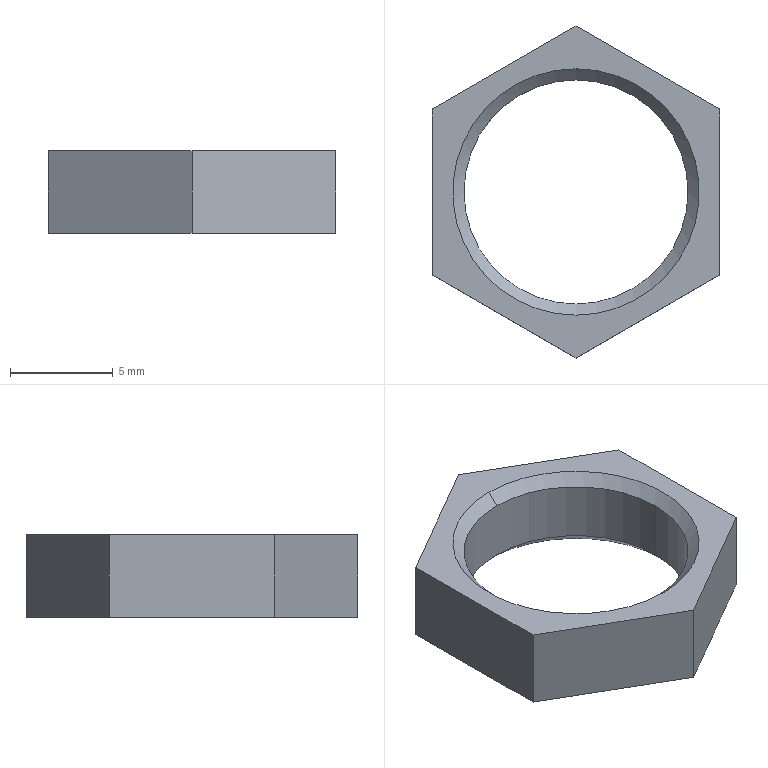Part | SolidWorks | features BaseBody 1 | 1 solid | 14 faces | box 14 x 16.166 x 4 mm | volume 294.157 mm3 | plane 8 | cone 4 | cylinder 2 | commonest cylinder face diameters 10.917 x2
STEP:
#1=CARTESIAN_POINT('',(-5.458,0.,-16.459));
#2=VERTEX_POINT('',#1);
#3=CARTESIAN_POINT('',(5.458,0.,-16.459));
#4=VERTEX_POINT('',#3);
#5=CARTESIAN_POINT('',(0.,0.,-16.459));
#6=DIRECTION('',(0.,0.,1.));
#7=DIRECTION('',(1.,0.,0.));
#8=AXIS2_PLACEMENT_3D('',#5,#6,#7);
#9=CIRCLE('',#8,5.458);
#10=EDGE_CURVE('',#2,#4,#9,.T.);
#11=ORIENTED_EDGE('',*,*,#10,.F.);
#12=CARTESIAN_POINT('',(-5.458,0.,-13.541));
#13=VERTEX_POINT('',#12);
#14=CARTESIAN_POINT('',(-5.458,0.,-50.));
#15=DIRECTION('',(0.,0.,1.));
#16=VECTOR('',#15,1000.);
#17=LINE('',#14,#16);
#18=EDGE_CURVE('',#2,#13,#17,.T.);
#19=ORIENTED_EDGE('',*,*,#18,.T.);
#20=CARTESIAN_POINT('',(0.,-5.458,-13.541));
#21=VERTEX_POINT('',#20);
#22=CARTESIAN_POINT('',(0.,0.,-13.541));
#23=DIRECTION('',(0.,0.,-1.));
#24=DIRECTION('',(1.,0.,0.));
#25=AXIS2_PLACEMENT_3D('',#22,#23,#24);
#26=CIRCLE('',#25,5.458);
#27=EDGE_CURVE('',#21,#13,#26,.T.);
#28=ORIENTED_EDGE('',*,*,#27,.F.);
#29=CARTESIAN_POINT('',(5.458,0.,-13.541));
#30=VERTEX_POINT('',#29);
#31=CARTESIAN_POINT('',(0.,0.,-13.541));
#32=DIRECTION('',(0.,0.,-1.));
#33=DIRECTION('',(1.,0.,0.));
#34=AXIS2_PLACEMENT_3D('',#31,#32,#33);
#35=CIRCLE('',#34,5.458);
#36=EDGE_CURVE('',#30,#21,#35,.T.);
#37=ORIENTED_EDGE('',*,*,#36,.F.);
#38=CARTESIAN_POINT('',(5.458,0.,-50.));
#39=DIRECTION('',(0.,0.,1.));
#40=VECTOR('',#39,1000.);
#41=LINE('',#38,#40);
#42=EDGE_CURVE('',#4,#30,#41,.T.);
#43=ORIENTED_EDGE('',*,*,#42,.F.);
#44=EDGE_LOOP('',(#11,#19,#28,#37,#43));
#45=FACE_OUTER_BOUND('',#44,.T.);
#46=CARTESIAN_POINT('',(0.,0.,-50.));
#47=DIRECTION('',(0.,0.,1.));
#48=DIRECTION('',(1.,0.,0.));
#49=AXIS2_PLACEMENT_3D('',#46,#47,#48);
#50=CYLINDRICAL_SURFACE('',#49,5.458);
#51=ADVANCED_FACE('',(#45),#50,.F.);
#52=ORIENTED_EDGE('',*,*,#27,.T.);
#53=CARTESIAN_POINT('',(0.,5.458,-13.541));
#54=VERTEX_POINT('',#53);
#55=CARTESIAN_POINT('',(0.,0.,-13.541));
#56=DIRECTION('',(0.,0.,-1.));
#57=DIRECTION('',(1.,0.,0.));
#58=AXIS2_PLACEMENT_3D('',#55,#56,#57);
#59=CIRCLE('',#58,5.458);
#60=EDGE_CURVE('',#13,#54,#59,.T.);
#61=ORIENTED_EDGE('',*,*,#60,.T.);
#62=CARTESIAN_POINT('',(0.,6.,-13.));
#63=VERTEX_POINT('',#62);
#64=CARTESIAN_POINT('',(0.,6.,-13.));
#65=DIRECTION('',(0.,0.7071,0.7071));
#66=VECTOR('',#65,1000.);
#67=LINE('',#64,#66);
#68=EDGE_CURVE('',#54,#63,#67,.T.);
#69=ORIENTED_EDGE('',*,*,#68,.T.);
#70=CARTESIAN_POINT('',(0.,-6.,-13.));
#71=VERTEX_POINT('',#70);
#72=CARTESIAN_POINT('',(0.,0.,-13.));
#73=DIRECTION('',(0.,0.,-1.));
#74=DIRECTION('',(0.,-1.,0.));
#75=AXIS2_PLACEMENT_3D('',#72,#73,#74);
#76=CIRCLE('',#75,6.);
#77=EDGE_CURVE('',#71,#63,#76,.T.);
#78=ORIENTED_EDGE('',*,*,#77,.F.);
#79=CARTESIAN_POINT('',(0.,-6.,-13.));
#80=DIRECTION('',(0.,-0.7071,0.7071));
#81=VECTOR('',#80,1000.);
#82=LINE('',#79,#81);
#83=EDGE_CURVE('',#21,#71,#82,.T.);
#84=ORIENTED_EDGE('',*,*,#83,.F.);
#85=EDGE_LOOP('',(#52,#61,#69,#78,#84));
#86=FACE_OUTER_BOUND('',#85,.T.);
#87=CARTESIAN_POINT('',(0.,0.,-13.));
#88=DIRECTION('',(0.,0.,1.));
#89=DIRECTION('',(0.,-1.,0.));
#90=AXIS2_PLACEMENT_3D('',#87,#88,#89);
#91=CONICAL_SURFACE('',#90,6.,0.7854);
#92=ADVANCED_FACE('',(#86),#91,.F.);
#93=ORIENTED_EDGE('',*,*,#10,.T.);
#94=CARTESIAN_POINT('',(6.,0.,-17.));
#95=VERTEX_POINT('',#94);
#96=CARTESIAN_POINT('',(6.,0.,-17.));
#97=DIRECTION('',(0.7071,0.,-0.7071));
#98=VECTOR('',#97,1000.);
#99=LINE('',#96,#98);
#100=EDGE_CURVE('',#4,#95,#99,.T.);
#101=ORIENTED_EDGE('',*,*,#100,.T.);
#102=CARTESIAN_POINT('',(-6.,0.,-17.));
#103=VERTEX_POINT('',#102);
#104=CARTESIAN_POINT('',(0.,0.,-17.));
#105=DIRECTION('',(0.,0.,1.));
#106=DIRECTION('',(-1.,0.,0.));
#107=AXIS2_PLACEMENT_3D('',#104,#105,#106);
#108=CIRCLE('',#107,6.);
#109=EDGE_CURVE('',#103,#95,#108,.T.);
#110=ORIENTED_EDGE('',*,*,#109,.F.);
#111=CARTESIAN_POINT('',(-6.,0.,-17.));
#112=DIRECTION('',(-0.7071,0.,-0.7071));
#113=VECTOR('',#112,1000.);
#114=LINE('',#111,#113);
#115=EDGE_CURVE('',#2,#103,#114,.T.);
#116=ORIENTED_EDGE('',*,*,#115,.F.);
#117=EDGE_LOOP('',(#93,#101,#110,#116));
#118=FACE_OUTER_BOUND('',#117,.T.);
#119=CARTESIAN_POINT('',(0.,0.,-17.));
#120=DIRECTION('',(0.,0.,-1.));
#121=DIRECTION('',(-1.,0.,0.));
#122=AXIS2_PLACEMENT_3D('',#119,#120,#121);
#123=CONICAL_SURFACE('',#122,6.,0.7854);
#124=ADVANCED_FACE('',(#118),#123,.F.);
#125=ORIENTED_EDGE('',*,*,#18,.F.);
#126=CARTESIAN_POINT('',(0.,0.,-16.459));
#127=DIRECTION('',(0.,0.,1.));
#128=DIRECTION('',(1.,0.,0.));
#129=AXIS2_PLACEMENT_3D('',#126,#127,#128);
#130=CIRCLE('',#129,5.458);
#131=EDGE_CURVE('',#4,#2,#130,.T.);
#132=ORIENTED_EDGE('',*,*,#131,.F.);
#133=ORIENTED_EDGE('',*,*,#42,.T.);
#134=CARTESIAN_POINT('',(0.,0.,-13.541));
#135=DIRECTION('',(0.,0.,-1.));
#136=DIRECTION('',(1.,0.,0.));
#137=AXIS2_PLACEMENT_3D('',#134,#135,#136);
#138=CIRCLE('',#137,5.458);
#139=EDGE_CURVE('',#54,#30,#138,.T.);
#140=ORIENTED_EDGE('',*,*,#139,.F.);
#141=ORIENTED_EDGE('',*,*,#60,.F.);
#142=EDGE_LOOP('',(#125,#132,#133,#140,#141));
#143=FACE_OUTER_BOUND('',#142,.T.);
#144=CARTESIAN_POINT('',(0.,0.,-50.));
#145=DIRECTION('',(0.,0.,1.));
#146=DIRECTION('',(1.,0.,0.));
#147=AXIS2_PLACEMENT_3D('',#144,#145,#146);
#148=CYLINDRICAL_SURFACE('',#147,5.458);
#149=ADVANCED_FACE('',(#143),#148,.F.);
#150=ORIENTED_EDGE('',*,*,#68,.F.);
#151=ORIENTED_EDGE('',*,*,#139,.T.);
#152=ORIENTED_EDGE('',*,*,#36,.T.);
#153=ORIENTED_EDGE('',*,*,#83,.T.);
#154=CARTESIAN_POINT('',(0.,0.,-13.));
#155=DIRECTION('',(0.,0.,-1.));
#156=DIRECTION('',(0.,-1.,0.));
#157=AXIS2_PLACEMENT_3D('',#154,#155,#156);
#158=CIRCLE('',#157,6.);
#159=EDGE_CURVE('',#63,#71,#158,.T.);
#160=ORIENTED_EDGE('',*,*,#159,.F.);
#161=EDGE_LOOP('',(#150,#151,#152,#153,#160));
#162=FACE_OUTER_BOUND('',#161,.T.);
#163=CARTESIAN_POINT('',(0.,0.,-13.));
#164=DIRECTION('',(0.,0.,1.));
#165=DIRECTION('',(0.,-1.,0.));
#166=AXIS2_PLACEMENT_3D('',#163,#164,#165);
#167=CONICAL_SURFACE('',#166,6.,0.7854);
#168=ADVANCED_FACE('',(#162),#167,.F.);
#169=ORIENTED_EDGE('',*,*,#100,.F.);
#170=ORIENTED_EDGE('',*,*,#131,.T.);
#171=ORIENTED_EDGE('',*,*,#115,.T.);
#172=CARTESIAN_POINT('',(0.,0.,-17.));
#173=DIRECTION('',(0.,0.,1.));
#174=DIRECTION('',(-1.,0.,0.));
#175=AXIS2_PLACEMENT_3D('',#172,#173,#174);
#176=CIRCLE('',#175,6.);
#177=EDGE_CURVE('',#95,#103,#176,.T.);
#178=ORIENTED_EDGE('',*,*,#177,.F.);
#179=EDGE_LOOP('',(#169,#170,#171,#178));
#180=FACE_OUTER_BOUND('',#179,.T.);
#181=CARTESIAN_POINT('',(0.,0.,-17.));
#182=DIRECTION('',(0.,0.,-1.));
#183=DIRECTION('',(-1.,0.,0.));
#184=AXIS2_PLACEMENT_3D('',#181,#182,#183);
#185=CONICAL_SURFACE('',#184,6.,0.7854);
#186=ADVANCED_FACE('',(#180),#185,.F.);
#187=ORIENTED_EDGE('',*,*,#77,.T.);
#188=ORIENTED_EDGE('',*,*,#159,.T.);
#189=EDGE_LOOP('',(#187,#188));
#190=FACE_BOUND('',#189,.T.);
#191=CARTESIAN_POINT('',(7.,-4.041,-13.));
#192=VERTEX_POINT('',#191);
#193=CARTESIAN_POINT('',(7.,4.041,-13.));
#194=VERTEX_POINT('',#193);
#195=CARTESIAN_POINT('',(7.,0.,-13.));
#196=DIRECTION('',(0.,1.,0.));
#197=VECTOR('',#196,1000.);
#198=LINE('',#195,#197);
#199=EDGE_CURVE('',#192,#194,#198,.T.);
#200=ORIENTED_EDGE('',*,*,#199,.T.);
#201=CARTESIAN_POINT('',(0.,8.083,-13.));
#202=VERTEX_POINT('',#201);
#203=CARTESIAN_POINT('',(7.,4.041,-13.));
#204=DIRECTION('',(-0.866,0.5,0.));
#205=VECTOR('',#204,1000.);
#206=LINE('',#203,#205);
#207=EDGE_CURVE('',#194,#202,#206,.T.);
#208=ORIENTED_EDGE('',*,*,#207,.T.);
#209=CARTESIAN_POINT('',(-7.,4.041,-13.));
#210=VERTEX_POINT('',#209);
#211=CARTESIAN_POINT('',(0.,8.083,-13.));
#212=DIRECTION('',(-0.866,-0.5,0.));
#213=VECTOR('',#212,1000.);
#214=LINE('',#211,#213);
#215=EDGE_CURVE('',#202,#210,#214,.T.);
#216=ORIENTED_EDGE('',*,*,#215,.T.);
#217=CARTESIAN_POINT('',(-7.,-4.041,-13.));
#218=VERTEX_POINT('',#217);
#219=CARTESIAN_POINT('',(-7.,0.,-13.));
#220=DIRECTION('',(0.,-1.,0.));
#221=VECTOR('',#220,1000.);
#222=LINE('',#219,#221);
#223=EDGE_CURVE('',#210,#218,#222,.T.);
#224=ORIENTED_EDGE('',*,*,#223,.T.);
#225=CARTESIAN_POINT('',(0.,-8.083,-13.));
#226=VERTEX_POINT('',#225);
#227=CARTESIAN_POINT('',(-7.,-4.041,-13.));
#228=DIRECTION('',(0.866,-0.5,0.));
#229=VECTOR('',#228,1000.);
#230=LINE('',#227,#229);
#231=EDGE_CURVE('',#218,#226,#230,.T.);
#232=ORIENTED_EDGE('',*,*,#231,.T.);
#233=CARTESIAN_POINT('',(0.,-8.083,-13.));
#234=DIRECTION('',(0.866,0.5,0.));
#235=VECTOR('',#234,1000.);
#236=LINE('',#233,#235);
#237=EDGE_CURVE('',#226,#192,#236,.T.);
#238=ORIENTED_EDGE('',*,*,#237,.T.);
#239=EDGE_LOOP('',(#200,#208,#216,#224,#232,#238));
#240=FACE_OUTER_BOUND('',#239,.T.);
#241=CARTESIAN_POINT('',(0.,0.,-13.));
#242=DIRECTION('',(0.,0.,1.));
#243=DIRECTION('',(1.,0.,0.));
#244=AXIS2_PLACEMENT_3D('',#241,#242,#243);
#245=PLANE('',#244);
#246=ADVANCED_FACE('',(#190,#240),#245,.T.);
#247=ORIENTED_EDGE('',*,*,#109,.T.);
#248=ORIENTED_EDGE('',*,*,#177,.T.);
#249=EDGE_LOOP('',(#247,#248));
#250=FACE_BOUND('',#249,.T.);
#251=CARTESIAN_POINT('',(7.,4.041,-17.));
#252=VERTEX_POINT('',#251);
#253=CARTESIAN_POINT('',(0.,8.083,-17.));
#254=VERTEX_POINT('',#253);
#255=CARTESIAN_POINT('',(7.,4.041,-17.));
#256=DIRECTION('',(-0.866,0.5,0.));
#257=VECTOR('',#256,1000.);
#258=LINE('',#255,#257);
#259=EDGE_CURVE('',#252,#254,#258,.T.);
#260=ORIENTED_EDGE('',*,*,#259,.F.);
#261=CARTESIAN_POINT('',(7.,-4.041,-17.));
#262=VERTEX_POINT('',#261);
#263=CARTESIAN_POINT('',(7.,0.,-17.));
#264=DIRECTION('',(0.,1.,0.));
#265=VECTOR('',#264,1000.);
#266=LINE('',#263,#265);
#267=EDGE_CURVE('',#262,#252,#266,.T.);
#268=ORIENTED_EDGE('',*,*,#267,.F.);
#269=CARTESIAN_POINT('',(0.,-8.083,-17.));
#270=VERTEX_POINT('',#269);
#271=CARTESIAN_POINT('',(0.,-8.083,-17.));
#272=DIRECTION('',(0.866,0.5,0.));
#273=VECTOR('',#272,1000.);
#274=LINE('',#271,#273);
#275=EDGE_CURVE('',#270,#262,#274,.T.);
#276=ORIENTED_EDGE('',*,*,#275,.F.);
#277=CARTESIAN_POINT('',(-7.,-4.041,-17.));
#278=VERTEX_POINT('',#277);
#279=CARTESIAN_POINT('',(-7.,-4.041,-17.));
#280=DIRECTION('',(0.866,-0.5,0.));
#281=VECTOR('',#280,1000.);
#282=LINE('',#279,#281);
#283=EDGE_CURVE('',#278,#270,#282,.T.);
#284=ORIENTED_EDGE('',*,*,#283,.F.);
#285=CARTESIAN_POINT('',(-7.,4.041,-17.));
#286=VERTEX_POINT('',#285);
#287=CARTESIAN_POINT('',(-7.,0.,-17.));
#288=DIRECTION('',(0.,-1.,0.));
#289=VECTOR('',#288,1000.);
#290=LINE('',#287,#289);
#291=EDGE_CURVE('',#286,#278,#290,.T.);
#292=ORIENTED_EDGE('',*,*,#291,.F.);
#293=CARTESIAN_POINT('',(0.,8.083,-17.));
#294=DIRECTION('',(-0.866,-0.5,0.));
#295=VECTOR('',#294,1000.);
#296=LINE('',#293,#295);
#297=EDGE_CURVE('',#254,#286,#296,.T.);
#298=ORIENTED_EDGE('',*,*,#297,.F.);
#299=EDGE_LOOP('',(#260,#268,#276,#284,#292,#298));
#300=FACE_OUTER_BOUND('',#299,.T.);
#301=CARTESIAN_POINT('',(0.,0.,-17.));
#302=DIRECTION('',(0.,0.,1.));
#303=DIRECTION('',(1.,0.,0.));
#304=AXIS2_PLACEMENT_3D('',#301,#302,#303);
#305=PLANE('',#304);
#306=ADVANCED_FACE('',(#250,#300),#305,.F.);
#307=ORIENTED_EDGE('',*,*,#259,.T.);
#308=CARTESIAN_POINT('',(0.,8.083,-17.));
#309=DIRECTION('',(0.,0.,1.));
#310=VECTOR('',#309,1000.);
#311=LINE('',#308,#310);
#312=EDGE_CURVE('',#254,#202,#311,.T.);
#313=ORIENTED_EDGE('',*,*,#312,.T.);
#314=ORIENTED_EDGE('',*,*,#207,.F.);
#315=CARTESIAN_POINT('',(7.,4.041,-17.));
#316=DIRECTION('',(0.,0.,-1.));
#317=VECTOR('',#316,1000.);
#318=LINE('',#315,#317);
#319=EDGE_CURVE('',#194,#252,#318,.T.);
#320=ORIENTED_EDGE('',*,*,#319,.T.);
#321=EDGE_LOOP('',(#307,#313,#314,#320));
#322=FACE_OUTER_BOUND('',#321,.T.);
#323=CARTESIAN_POINT('',(7.,4.041,-17.));
#324=DIRECTION('',(0.5,0.866,0.));
#325=DIRECTION('',(-0.866,0.5,0.));
#326=AXIS2_PLACEMENT_3D('',#323,#324,#325);
#327=PLANE('',#326);
#328=ADVANCED_FACE('',(#322),#327,.T.);
#329=ORIENTED_EDGE('',*,*,#267,.T.);
#330=ORIENTED_EDGE('',*,*,#319,.F.);
#331=ORIENTED_EDGE('',*,*,#199,.F.);
#332=CARTESIAN_POINT('',(7.,-4.041,-17.));
#333=DIRECTION('',(0.,0.,-1.));
#334=VECTOR('',#333,1000.);
#335=LINE('',#332,#334);
#336=EDGE_CURVE('',#192,#262,#335,.T.);
#337=ORIENTED_EDGE('',*,*,#336,.T.);
#338=EDGE_LOOP('',(#329,#330,#331,#337));
#339=FACE_OUTER_BOUND('',#338,.T.);
#340=CARTESIAN_POINT('',(7.,-4.041,-17.));
#341=DIRECTION('',(1.,0.,0.));
#342=DIRECTION('',(0.,0.,-1.));
#343=AXIS2_PLACEMENT_3D('',#340,#341,#342);
#344=PLANE('',#343);
#345=ADVANCED_FACE('',(#339),#344,.T.);
#346=ORIENTED_EDGE('',*,*,#275,.T.);
#347=ORIENTED_EDGE('',*,*,#336,.F.);
#348=ORIENTED_EDGE('',*,*,#237,.F.);
#349=CARTESIAN_POINT('',(0.,-8.083,-17.));
#350=DIRECTION('',(0.,0.,-1.));
#351=VECTOR('',#350,1000.);
#352=LINE('',#349,#351);
#353=EDGE_CURVE('',#226,#270,#352,.T.);
#354=ORIENTED_EDGE('',*,*,#353,.T.);
#355=EDGE_LOOP('',(#346,#347,#348,#354));
#356=FACE_OUTER_BOUND('',#355,.T.);
#357=CARTESIAN_POINT('',(0.,-8.083,-17.));
#358=DIRECTION('',(0.5,-0.866,0.));
#359=DIRECTION('',(0.866,0.5,0.));
#360=AXIS2_PLACEMENT_3D('',#357,#358,#359);
#361=PLANE('',#360);
#362=ADVANCED_FACE('',(#356),#361,.T.);
#363=ORIENTED_EDGE('',*,*,#283,.T.);
#364=ORIENTED_EDGE('',*,*,#353,.F.);
#365=ORIENTED_EDGE('',*,*,#231,.F.);
#366=CARTESIAN_POINT('',(-7.,-4.041,-17.));
#367=DIRECTION('',(0.,0.,-1.));
#368=VECTOR('',#367,1000.);
#369=LINE('',#366,#368);
#370=EDGE_CURVE('',#218,#278,#369,.T.);
#371=ORIENTED_EDGE('',*,*,#370,.T.);
#372=EDGE_LOOP('',(#363,#364,#365,#371));
#373=FACE_OUTER_BOUND('',#372,.T.);
#374=CARTESIAN_POINT('',(-7.,-4.041,-17.));
#375=DIRECTION('',(-0.5,-0.866,0.));
#376=DIRECTION('',(0.866,-0.5,0.));
#377=AXIS2_PLACEMENT_3D('',#374,#375,#376);
#378=PLANE('',#377);
#379=ADVANCED_FACE('',(#373),#378,.T.);
#380=ORIENTED_EDGE('',*,*,#291,.T.);
#381=ORIENTED_EDGE('',*,*,#370,.F.);
#382=ORIENTED_EDGE('',*,*,#223,.F.);
#383=CARTESIAN_POINT('',(-7.,4.041,-17.));
#384=DIRECTION('',(0.,0.,-1.));
#385=VECTOR('',#384,1000.);
#386=LINE('',#383,#385);
#387=EDGE_CURVE('',#210,#286,#386,.T.);
#388=ORIENTED_EDGE('',*,*,#387,.T.);
#389=EDGE_LOOP('',(#380,#381,#382,#388));
#390=FACE_OUTER_BOUND('',#389,.T.);
#391=CARTESIAN_POINT('',(-7.,4.041,-17.));
#392=DIRECTION('',(-1.,0.,0.));
#393=DIRECTION('',(0.,0.,1.));
#394=AXIS2_PLACEMENT_3D('',#391,#392,#393);
#395=PLANE('',#394);
#396=ADVANCED_FACE('',(#390),#395,.T.);
#397=ORIENTED_EDGE('',*,*,#297,.T.);
#398=ORIENTED_EDGE('',*,*,#387,.F.);
#399=ORIENTED_EDGE('',*,*,#215,.F.);
#400=ORIENTED_EDGE('',*,*,#312,.F.);
#401=EDGE_LOOP('',(#397,#398,#399,#400));
#402=FACE_OUTER_BOUND('',#401,.T.);
#403=CARTESIAN_POINT('',(0.,8.083,-17.));
#404=DIRECTION('',(-0.5,0.866,0.));
#405=DIRECTION('',(-0.866,-0.5,0.));
#406=AXIS2_PLACEMENT_3D('',#403,#404,#405);
#407=PLANE('',#406);
#408=ADVANCED_FACE('',(#402),#407,.T.);
#409=CLOSED_SHELL('',(#51,#92,#124,#149,#168,#186,#246,#306,#328,#345,#362,#379,#396,#408));
#410=MANIFOLD_SOLID_BREP('',#409);
#411=CARTESIAN_POINT('',(0.,0.,0.));
#412=DIRECTION('',(0.,0.,1.));
#413=DIRECTION('',(1.,0.,0.));
#414=AXIS2_PLACEMENT_3D('',#411,#412,#413);
#415=(LENGTH_UNIT()NAMED_UNIT(*)SI_UNIT(.MILLI.,.METRE.));
#416=UNCERTAINTY_MEASURE_WITH_UNIT(LENGTH_MEASURE(0.00001),#415,'','');
#417=(NAMED_UNIT(*)PLANE_ANGLE_UNIT()SI_UNIT($,.RADIAN.));
#418=(NAMED_UNIT(*)SI_UNIT($,.STERADIAN.)SOLID_ANGLE_UNIT());
#419=(GEOMETRIC_REPRESENTATION_CONTEXT(3)GLOBAL_UNCERTAINTY_ASSIGNED_CONTEXT((#416))GLOBAL_UNIT_ASSIGNED_CONTEXT((#415,#417,#418))REPRESENTATION_CONTEXT('',''));
#420=ADVANCED_BREP_SHAPE_REPRESENTATION('',(#410,#414),#419);